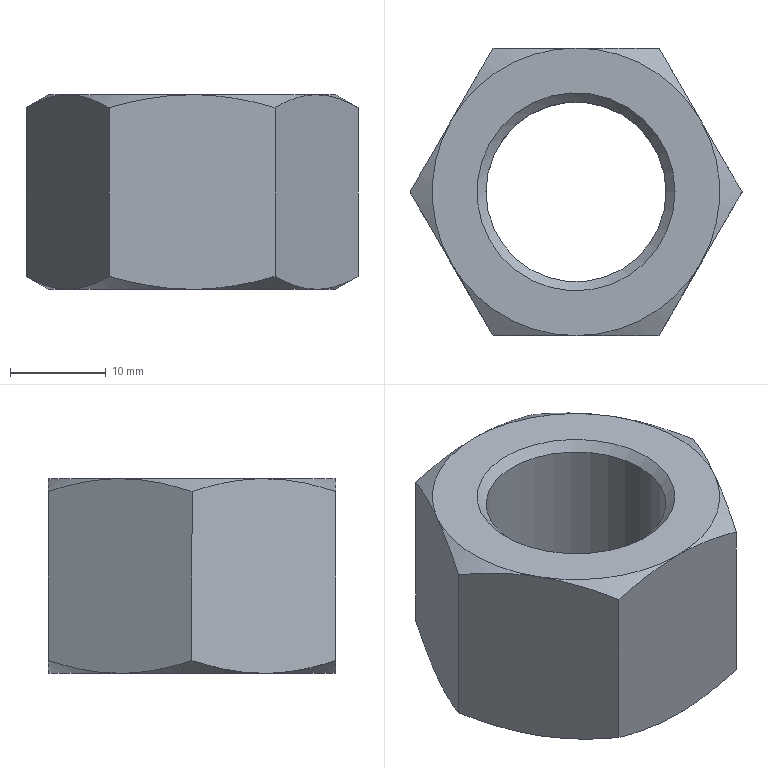Part | NX | features META 3, SKETCH 3, DATUM_CSYS 2, EXTRUDE 2, SWP104 2, CHAMFER 1, LINE 1, SYMBOLIC_THREAD 1, THREADS 1 | 1 solid | 23 faces | box 34.641 x 30 x 20.3 mm | volume 10084 mm3 | cone 14 | plane 8 | cylinder 1 | commonest cylinder face diameters 18.782 x1
STEP:
#1=CARTESIAN_POINT('',(10.33,0.,20.3));
#2=VERTEX_POINT('',#1);
#3=CARTESIAN_POINT('',(0.,0.,20.3));
#4=DIRECTION('',(0.,0.,1.));
#5=DIRECTION('',(1.,0.,0.));
#6=AXIS2_PLACEMENT_3D('',#3,#4,#5);
#7=CIRCLE('',#6,10.33);
#8=EDGE_CURVE('',#2,#2,#7,.F.);
#9=ORIENTED_EDGE('',*,*,#8,.T.);
#10=EDGE_LOOP('',(#9));
#11=FACE_BOUND('',#10,.T.);
#12=CARTESIAN_POINT('',(-12.99,7.5,20.3));
#13=VERTEX_POINT('',#12);
#14=CARTESIAN_POINT('',(0.,15.,20.3));
#15=VERTEX_POINT('',#14);
#16=CARTESIAN_POINT('',(0.,0.,20.3));
#17=DIRECTION('',(0.,0.,-1.));
#18=DIRECTION('',(-1.,0.,0.));
#19=AXIS2_PLACEMENT_3D('',#16,#17,#18);
#20=CIRCLE('',#19,15.);
#21=EDGE_CURVE('',#13,#15,#20,.T.);
#22=ORIENTED_EDGE('',*,*,#21,.F.);
#23=CARTESIAN_POINT('',(-12.99,-7.5,20.3));
#24=VERTEX_POINT('',#23);
#25=CARTESIAN_POINT('',(0.,0.,20.3));
#26=DIRECTION('',(0.,0.,-1.));
#27=DIRECTION('',(-1.,0.,0.));
#28=AXIS2_PLACEMENT_3D('',#25,#26,#27);
#29=CIRCLE('',#28,15.);
#30=EDGE_CURVE('',#24,#13,#29,.T.);
#31=ORIENTED_EDGE('',*,*,#30,.F.);
#32=CARTESIAN_POINT('',(0.,-15.,20.3));
#33=VERTEX_POINT('',#32);
#34=CARTESIAN_POINT('',(0.,0.,20.3));
#35=DIRECTION('',(0.,0.,-1.));
#36=DIRECTION('',(-1.,0.,0.));
#37=AXIS2_PLACEMENT_3D('',#34,#35,#36);
#38=CIRCLE('',#37,15.);
#39=EDGE_CURVE('',#33,#24,#38,.T.);
#40=ORIENTED_EDGE('',*,*,#39,.F.);
#41=CARTESIAN_POINT('',(12.99,-7.5,20.3));
#42=VERTEX_POINT('',#41);
#43=CARTESIAN_POINT('',(0.,0.,20.3));
#44=DIRECTION('',(0.,0.,-1.));
#45=DIRECTION('',(-1.,0.,0.));
#46=AXIS2_PLACEMENT_3D('',#43,#44,#45);
#47=CIRCLE('',#46,15.);
#48=EDGE_CURVE('',#42,#33,#47,.T.);
#49=ORIENTED_EDGE('',*,*,#48,.F.);
#50=CARTESIAN_POINT('',(12.99,7.5,20.3));
#51=VERTEX_POINT('',#50);
#52=CARTESIAN_POINT('',(0.,0.,20.3));
#53=DIRECTION('',(0.,0.,-1.));
#54=DIRECTION('',(-1.,0.,0.));
#55=AXIS2_PLACEMENT_3D('',#52,#53,#54);
#56=CIRCLE('',#55,15.);
#57=EDGE_CURVE('',#51,#42,#56,.T.);
#58=ORIENTED_EDGE('',*,*,#57,.F.);
#59=CARTESIAN_POINT('',(0.,0.,20.3));
#60=DIRECTION('',(0.,0.,-1.));
#61=DIRECTION('',(-1.,0.,0.));
#62=AXIS2_PLACEMENT_3D('',#59,#60,#61);
#63=CIRCLE('',#62,15.);
#64=EDGE_CURVE('',#15,#51,#63,.T.);
#65=ORIENTED_EDGE('',*,*,#64,.F.);
#66=EDGE_LOOP('',(#22,#31,#40,#49,#58,#65));
#67=FACE_BOUND('',#66,.T.);
#68=CARTESIAN_POINT('',(0.,30.,20.3));
#69=DIRECTION('',(0.,0.,1.));
#70=DIRECTION('',(1.,0.,0.));
#71=AXIS2_PLACEMENT_3D('',#68,#69,#70);
#72=PLANE('',#71);
#73=ADVANCED_FACE('',(#11,#67),#72,.T.);
#74=CARTESIAN_POINT('',(10.33,0.,0.));
#75=VERTEX_POINT('',#74);
#76=CARTESIAN_POINT('',(0.,0.,0.));
#77=DIRECTION('',(0.,0.,1.));
#78=DIRECTION('',(1.,0.,0.));
#79=AXIS2_PLACEMENT_3D('',#76,#77,#78);
#80=CIRCLE('',#79,10.33);
#81=EDGE_CURVE('',#75,#75,#80,.T.);
#82=ORIENTED_EDGE('',*,*,#81,.T.);
#83=EDGE_LOOP('',(#82));
#84=FACE_BOUND('',#83,.T.);
#85=CARTESIAN_POINT('',(-12.99,-7.5,0.));
#86=VERTEX_POINT('',#85);
#87=CARTESIAN_POINT('',(-12.99,7.5,0.));
#88=VERTEX_POINT('',#87);
#89=CARTESIAN_POINT('',(0.,0.,0.));
#90=DIRECTION('',(0.,0.,-1.));
#91=DIRECTION('',(-1.,0.,0.));
#92=AXIS2_PLACEMENT_3D('',#89,#90,#91);
#93=CIRCLE('',#92,15.);
#94=EDGE_CURVE('',#86,#88,#93,.T.);
#95=ORIENTED_EDGE('',*,*,#94,.T.);
#96=CARTESIAN_POINT('',(0.,15.,0.));
#97=VERTEX_POINT('',#96);
#98=CARTESIAN_POINT('',(0.,0.,0.));
#99=DIRECTION('',(0.,0.,-1.));
#100=DIRECTION('',(-1.,0.,0.));
#101=AXIS2_PLACEMENT_3D('',#98,#99,#100);
#102=CIRCLE('',#101,15.);
#103=EDGE_CURVE('',#88,#97,#102,.T.);
#104=ORIENTED_EDGE('',*,*,#103,.T.);
#105=CARTESIAN_POINT('',(12.99,7.5,0.));
#106=VERTEX_POINT('',#105);
#107=CARTESIAN_POINT('',(0.,0.,0.));
#108=DIRECTION('',(0.,0.,-1.));
#109=DIRECTION('',(-1.,0.,0.));
#110=AXIS2_PLACEMENT_3D('',#107,#108,#109);
#111=CIRCLE('',#110,15.);
#112=EDGE_CURVE('',#97,#106,#111,.T.);
#113=ORIENTED_EDGE('',*,*,#112,.T.);
#114=CARTESIAN_POINT('',(12.99,-7.5,0.));
#115=VERTEX_POINT('',#114);
#116=CARTESIAN_POINT('',(0.,0.,0.));
#117=DIRECTION('',(0.,0.,-1.));
#118=DIRECTION('',(-1.,0.,0.));
#119=AXIS2_PLACEMENT_3D('',#116,#117,#118);
#120=CIRCLE('',#119,15.);
#121=EDGE_CURVE('',#106,#115,#120,.T.);
#122=ORIENTED_EDGE('',*,*,#121,.T.);
#123=CARTESIAN_POINT('',(0.,-15.,0.));
#124=VERTEX_POINT('',#123);
#125=CARTESIAN_POINT('',(0.,0.,0.));
#126=DIRECTION('',(0.,0.,-1.));
#127=DIRECTION('',(-1.,0.,0.));
#128=AXIS2_PLACEMENT_3D('',#125,#126,#127);
#129=CIRCLE('',#128,15.);
#130=EDGE_CURVE('',#115,#124,#129,.T.);
#131=ORIENTED_EDGE('',*,*,#130,.T.);
#132=CARTESIAN_POINT('',(0.,0.,0.));
#133=DIRECTION('',(0.,0.,-1.));
#134=DIRECTION('',(-1.,0.,0.));
#135=AXIS2_PLACEMENT_3D('',#132,#133,#134);
#136=CIRCLE('',#135,15.);
#137=EDGE_CURVE('',#124,#86,#136,.T.);
#138=ORIENTED_EDGE('',*,*,#137,.T.);
#139=EDGE_LOOP('',(#95,#104,#113,#122,#131,#138));
#140=FACE_BOUND('',#139,.T.);
#141=CARTESIAN_POINT('',(0.,30.,0.));
#142=DIRECTION('',(0.,0.,1.));
#143=DIRECTION('',(1.,0.,0.));
#144=AXIS2_PLACEMENT_3D('',#141,#142,#143);
#145=PLANE('',#144);
#146=ADVANCED_FACE('',(#84,#140),#145,.F.);
#147=CARTESIAN_POINT('',(17.321,0.,18.96));
#148=VERTEX_POINT('',#147);
#149=CARTESIAN_POINT('',(17.321,0.,1.34));
#150=VERTEX_POINT('',#149);
#151=CARTESIAN_POINT('',(17.321,0.,20.3));
#152=DIRECTION('',(0.,0.,-1.));
#153=VECTOR('',#152,1000.);
#154=LINE('',#151,#153);
#155=EDGE_CURVE('',#148,#150,#154,.T.);
#156=ORIENTED_EDGE('',*,*,#155,.T.);
#157=CARTESIAN_POINT('',(17.321,0.,1.34));
#158=CARTESIAN_POINT('',(15.904,2.454,0.5218));
#159=CARTESIAN_POINT('',(14.466,4.944,0.));
#160=CARTESIAN_POINT('',(12.99,7.5,0.));
#161=B_SPLINE_CURVE_WITH_KNOTS('',3,(#157,#158,#159,#160),.UNSPECIFIED.,.F.,.F.,(4,4),(0.000000238,0.008763),.UNSPECIFIED.);
#162=EDGE_CURVE('',#150,#106,#161,.T.);
#163=ORIENTED_EDGE('',*,*,#162,.T.);
#164=CARTESIAN_POINT('',(8.66,15.,1.34));
#165=VERTEX_POINT('',#164);
#166=CARTESIAN_POINT('',(12.99,7.5,0.));
#167=CARTESIAN_POINT('',(11.52,10.046,0.));
#168=CARTESIAN_POINT('',(10.073,12.552,0.5239));
#169=CARTESIAN_POINT('',(8.66,15.,1.34));
#170=B_SPLINE_CURVE_WITH_KNOTS('',3,(#166,#167,#168,#169),.UNSPECIFIED.,.F.,.F.,(4,4),(0.008763,0.01749),.UNSPECIFIED.);
#171=EDGE_CURVE('',#106,#165,#170,.T.);
#172=ORIENTED_EDGE('',*,*,#171,.T.);
#173=CARTESIAN_POINT('',(8.66,15.,18.96));
#174=VERTEX_POINT('',#173);
#175=CARTESIAN_POINT('',(8.66,15.,20.3));
#176=DIRECTION('',(0.,0.,-1.));
#177=VECTOR('',#176,1000.);
#178=LINE('',#175,#177);
#179=EDGE_CURVE('',#174,#165,#178,.T.);
#180=ORIENTED_EDGE('',*,*,#179,.F.);
#181=CARTESIAN_POINT('',(8.66,15.,18.96));
#182=CARTESIAN_POINT('',(10.077,12.546,19.778));
#183=CARTESIAN_POINT('',(11.515,10.056,20.3));
#184=CARTESIAN_POINT('',(12.99,7.5,20.3));
#185=B_SPLINE_CURVE_WITH_KNOTS('',3,(#181,#182,#183,#184),.UNSPECIFIED.,.F.,.F.,(4,4),(0.000000238,0.008763),.UNSPECIFIED.);
#186=EDGE_CURVE('',#174,#51,#185,.T.);
#187=ORIENTED_EDGE('',*,*,#186,.T.);
#188=CARTESIAN_POINT('',(12.99,7.5,20.3));
#189=CARTESIAN_POINT('',(14.46,4.954,20.3));
#190=CARTESIAN_POINT('',(15.907,2.448,19.776));
#191=CARTESIAN_POINT('',(17.321,0.,18.96));
#192=B_SPLINE_CURVE_WITH_KNOTS('',3,(#188,#189,#190,#191),.UNSPECIFIED.,.F.,.F.,(4,4),(0.008763,0.01749),.UNSPECIFIED.);
#193=EDGE_CURVE('',#51,#148,#192,.T.);
#194=ORIENTED_EDGE('',*,*,#193,.T.);
#195=EDGE_LOOP('',(#156,#163,#172,#180,#187,#194));
#196=FACE_BOUND('',#195,.T.);
#197=CARTESIAN_POINT('',(8.66,15.,20.3));
#198=DIRECTION('',(0.866,0.5,0.));
#199=DIRECTION('',(-0.5,0.866,0.));
#200=AXIS2_PLACEMENT_3D('',#197,#198,#199);
#201=PLANE('',#200);
#202=ADVANCED_FACE('',(#196),#201,.T.);
#203=CARTESIAN_POINT('',(8.66,-15.,18.96));
#204=VERTEX_POINT('',#203);
#205=CARTESIAN_POINT('',(8.66,-15.,1.34));
#206=VERTEX_POINT('',#205);
#207=CARTESIAN_POINT('',(8.66,-15.,20.3));
#208=DIRECTION('',(0.,0.,-1.));
#209=VECTOR('',#208,1000.);
#210=LINE('',#207,#209);
#211=EDGE_CURVE('',#204,#206,#210,.T.);
#212=ORIENTED_EDGE('',*,*,#211,.T.);
#213=CARTESIAN_POINT('',(8.66,-15.,1.34));
#214=CARTESIAN_POINT('',(10.077,-12.546,0.5218));
#215=CARTESIAN_POINT('',(11.515,-10.056,0.));
#216=CARTESIAN_POINT('',(12.99,-7.5,0.));
#217=B_SPLINE_CURVE_WITH_KNOTS('',3,(#213,#214,#215,#216),.UNSPECIFIED.,.F.,.F.,(4,4),(0.000000238,0.008763),.UNSPECIFIED.);
#218=EDGE_CURVE('',#206,#115,#217,.T.);
#219=ORIENTED_EDGE('',*,*,#218,.T.);
#220=CARTESIAN_POINT('',(12.99,-7.5,0.));
#221=CARTESIAN_POINT('',(14.46,-4.954,0.));
#222=CARTESIAN_POINT('',(15.907,-2.448,0.5239));
#223=CARTESIAN_POINT('',(17.321,0.,1.34));
#224=B_SPLINE_CURVE_WITH_KNOTS('',3,(#220,#221,#222,#223),.UNSPECIFIED.,.F.,.F.,(4,4),(0.008763,0.01749),.UNSPECIFIED.);
#225=EDGE_CURVE('',#115,#150,#224,.T.);
#226=ORIENTED_EDGE('',*,*,#225,.T.);
#227=ORIENTED_EDGE('',*,*,#155,.F.);
#228=CARTESIAN_POINT('',(17.321,0.,18.96));
#229=CARTESIAN_POINT('',(15.904,-2.454,19.778));
#230=CARTESIAN_POINT('',(14.466,-4.944,20.3));
#231=CARTESIAN_POINT('',(12.99,-7.5,20.3));
#232=B_SPLINE_CURVE_WITH_KNOTS('',3,(#228,#229,#230,#231),.UNSPECIFIED.,.F.,.F.,(4,4),(0.000000238,0.008763),.UNSPECIFIED.);
#233=EDGE_CURVE('',#148,#42,#232,.T.);
#234=ORIENTED_EDGE('',*,*,#233,.T.);
#235=CARTESIAN_POINT('',(12.99,-7.5,20.3));
#236=CARTESIAN_POINT('',(11.52,-10.046,20.3));
#237=CARTESIAN_POINT('',(10.073,-12.552,19.776));
#238=CARTESIAN_POINT('',(8.66,-15.,18.96));
#239=B_SPLINE_CURVE_WITH_KNOTS('',3,(#235,#236,#237,#238),.UNSPECIFIED.,.F.,.F.,(4,4),(0.008763,0.01749),.UNSPECIFIED.);
#240=EDGE_CURVE('',#42,#204,#239,.T.);
#241=ORIENTED_EDGE('',*,*,#240,.T.);
#242=EDGE_LOOP('',(#212,#219,#226,#227,#234,#241));
#243=FACE_BOUND('',#242,.T.);
#244=CARTESIAN_POINT('',(17.321,0.,20.3));
#245=DIRECTION('',(0.866,-0.5,0.));
#246=DIRECTION('',(0.5,0.866,0.));
#247=AXIS2_PLACEMENT_3D('',#244,#245,#246);
#248=PLANE('',#247);
#249=ADVANCED_FACE('',(#243),#248,.T.);
#250=CARTESIAN_POINT('',(-8.66,-15.,18.96));
#251=VERTEX_POINT('',#250);
#252=CARTESIAN_POINT('',(-8.66,-15.,1.34));
#253=VERTEX_POINT('',#252);
#254=CARTESIAN_POINT('',(-8.66,-15.,20.3));
#255=DIRECTION('',(0.,0.,-1.));
#256=VECTOR('',#255,1000.);
#257=LINE('',#254,#256);
#258=EDGE_CURVE('',#251,#253,#257,.T.);
#259=ORIENTED_EDGE('',*,*,#258,.T.);
#260=CARTESIAN_POINT('',(-8.66,-15.,1.34));
#261=CARTESIAN_POINT('',(-5.843,-15.,0.5265));
#262=CARTESIAN_POINT('',(-2.927,-15.,0.));
#263=CARTESIAN_POINT('',(0.,-15.,0.));
#264=B_SPLINE_CURVE_WITH_KNOTS('',3,(#260,#261,#262,#263),.UNSPECIFIED.,.F.,.F.,(4,4),(0.01545,0.02421),.UNSPECIFIED.);
#265=EDGE_CURVE('',#253,#124,#264,.T.);
#266=ORIENTED_EDGE('',*,*,#265,.T.);
#267=CARTESIAN_POINT('',(0.,-15.,0.));
#268=CARTESIAN_POINT('',(2.929,-15.,0.));
#269=CARTESIAN_POINT('',(5.86,-15.,0.5313));
#270=CARTESIAN_POINT('',(8.66,-15.,1.34));
#271=B_SPLINE_CURVE_WITH_KNOTS('',3,(#267,#268,#269,#270),.UNSPECIFIED.,.F.,.F.,(4,4),(0.02421,0.03298),.UNSPECIFIED.);
#272=EDGE_CURVE('',#124,#206,#271,.T.);
#273=ORIENTED_EDGE('',*,*,#272,.T.);
#274=ORIENTED_EDGE('',*,*,#211,.F.);
#275=CARTESIAN_POINT('',(0.,-15.,20.3));
#276=CARTESIAN_POINT('',(2.929,-15.,20.3));
#277=CARTESIAN_POINT('',(5.86,-15.,19.769));
#278=CARTESIAN_POINT('',(8.66,-15.,18.96));
#279=B_SPLINE_CURVE_WITH_KNOTS('',3,(#275,#276,#277,#278),.UNSPECIFIED.,.F.,.F.,(4,4),(0.02421,0.03298),.UNSPECIFIED.);
#280=EDGE_CURVE('',#204,#33,#279,.F.);
#281=ORIENTED_EDGE('',*,*,#280,.T.);
#282=CARTESIAN_POINT('',(-8.66,-15.,18.96));
#283=CARTESIAN_POINT('',(-5.843,-15.,19.773));
#284=CARTESIAN_POINT('',(-2.927,-15.,20.3));
#285=CARTESIAN_POINT('',(0.,-15.,20.3));
#286=B_SPLINE_CURVE_WITH_KNOTS('',3,(#282,#283,#284,#285),.UNSPECIFIED.,.F.,.F.,(4,4),(0.01545,0.02421),.UNSPECIFIED.);
#287=EDGE_CURVE('',#33,#251,#286,.F.);
#288=ORIENTED_EDGE('',*,*,#287,.T.);
#289=EDGE_LOOP('',(#259,#266,#273,#274,#281,#288));
#290=FACE_BOUND('',#289,.T.);
#291=CARTESIAN_POINT('',(8.66,-15.,20.3));
#292=DIRECTION('',(0.,-1.,0.));
#293=DIRECTION('',(1.,0.,0.));
#294=AXIS2_PLACEMENT_3D('',#291,#292,#293);
#295=PLANE('',#294);
#296=ADVANCED_FACE('',(#290),#295,.T.);
#297=CARTESIAN_POINT('',(-17.321,0.,18.96));
#298=VERTEX_POINT('',#297);
#299=CARTESIAN_POINT('',(-17.321,0.,1.34));
#300=VERTEX_POINT('',#299);
#301=CARTESIAN_POINT('',(-17.321,0.,20.3));
#302=DIRECTION('',(0.,0.,-1.));
#303=VECTOR('',#302,1000.);
#304=LINE('',#301,#303);
#305=EDGE_CURVE('',#298,#300,#304,.T.);
#306=ORIENTED_EDGE('',*,*,#305,.T.);
#307=CARTESIAN_POINT('',(-17.321,0.,1.34));
#308=CARTESIAN_POINT('',(-15.904,-2.454,0.5218));
#309=CARTESIAN_POINT('',(-14.466,-4.944,0.));
#310=CARTESIAN_POINT('',(-12.99,-7.5,0.));
#311=B_SPLINE_CURVE_WITH_KNOTS('',3,(#307,#308,#309,#310),.UNSPECIFIED.,.F.,.F.,(4,4),(0.000000238,0.008763),.UNSPECIFIED.);
#312=EDGE_CURVE('',#300,#86,#311,.T.);
#313=ORIENTED_EDGE('',*,*,#312,.T.);
#314=CARTESIAN_POINT('',(-12.99,-7.5,0.));
#315=CARTESIAN_POINT('',(-11.52,-10.046,0.));
#316=CARTESIAN_POINT('',(-10.073,-12.552,0.5239));
#317=CARTESIAN_POINT('',(-8.66,-15.,1.34));
#318=B_SPLINE_CURVE_WITH_KNOTS('',3,(#314,#315,#316,#317),.UNSPECIFIED.,.F.,.F.,(4,4),(0.008763,0.01749),.UNSPECIFIED.);
#319=EDGE_CURVE('',#86,#253,#318,.T.);
#320=ORIENTED_EDGE('',*,*,#319,.T.);
#321=ORIENTED_EDGE('',*,*,#258,.F.);
#322=CARTESIAN_POINT('',(-8.66,-15.,18.96));
#323=CARTESIAN_POINT('',(-10.077,-12.546,19.778));
#324=CARTESIAN_POINT('',(-11.515,-10.056,20.3));
#325=CARTESIAN_POINT('',(-12.99,-7.5,20.3));
#326=B_SPLINE_CURVE_WITH_KNOTS('',3,(#322,#323,#324,#325),.UNSPECIFIED.,.F.,.F.,(4,4),(0.000000238,0.008763),.UNSPECIFIED.);
#327=EDGE_CURVE('',#251,#24,#326,.T.);
#328=ORIENTED_EDGE('',*,*,#327,.T.);
#329=CARTESIAN_POINT('',(-12.99,-7.5,20.3));
#330=CARTESIAN_POINT('',(-14.46,-4.954,20.3));
#331=CARTESIAN_POINT('',(-15.907,-2.448,19.776));
#332=CARTESIAN_POINT('',(-17.321,0.,18.96));
#333=B_SPLINE_CURVE_WITH_KNOTS('',3,(#329,#330,#331,#332),.UNSPECIFIED.,.F.,.F.,(4,4),(0.008763,0.01749),.UNSPECIFIED.);
#334=EDGE_CURVE('',#24,#298,#333,.T.);
#335=ORIENTED_EDGE('',*,*,#334,.T.);
#336=EDGE_LOOP('',(#306,#313,#320,#321,#328,#335));
#337=FACE_BOUND('',#336,.T.);
#338=CARTESIAN_POINT('',(-8.66,-15.,20.3));
#339=DIRECTION('',(-0.866,-0.5,0.));
#340=DIRECTION('',(0.5,-0.866,0.));
#341=AXIS2_PLACEMENT_3D('',#338,#339,#340);
#342=PLANE('',#341);
#343=ADVANCED_FACE('',(#337),#342,.T.);
#344=CARTESIAN_POINT('',(-8.66,15.,18.96));
#345=VERTEX_POINT('',#344);
#346=CARTESIAN_POINT('',(-8.66,15.,1.34));
#347=VERTEX_POINT('',#346);
#348=CARTESIAN_POINT('',(-8.66,15.,20.3));
#349=DIRECTION('',(0.,0.,-1.));
#350=VECTOR('',#349,1000.);
#351=LINE('',#348,#350);
#352=EDGE_CURVE('',#345,#347,#351,.T.);
#353=ORIENTED_EDGE('',*,*,#352,.T.);
#354=CARTESIAN_POINT('',(-8.66,15.,1.34));
#355=CARTESIAN_POINT('',(-10.077,12.546,0.5218));
#356=CARTESIAN_POINT('',(-11.515,10.056,0.));
#357=CARTESIAN_POINT('',(-12.99,7.5,0.));
#358=B_SPLINE_CURVE_WITH_KNOTS('',3,(#354,#355,#356,#357),.UNSPECIFIED.,.F.,.F.,(4,4),(0.000000238,0.008763),.UNSPECIFIED.);
#359=EDGE_CURVE('',#347,#88,#358,.T.);
#360=ORIENTED_EDGE('',*,*,#359,.T.);
#361=CARTESIAN_POINT('',(-12.99,7.5,0.));
#362=CARTESIAN_POINT('',(-14.46,4.954,0.));
#363=CARTESIAN_POINT('',(-15.907,2.448,0.5239));
#364=CARTESIAN_POINT('',(-17.321,0.,1.34));
#365=B_SPLINE_CURVE_WITH_KNOTS('',3,(#361,#362,#363,#364),.UNSPECIFIED.,.F.,.F.,(4,4),(0.008763,0.01749),.UNSPECIFIED.);
#366=EDGE_CURVE('',#88,#300,#365,.T.);
#367=ORIENTED_EDGE('',*,*,#366,.T.);
#368=ORIENTED_EDGE('',*,*,#305,.F.);
#369=CARTESIAN_POINT('',(-17.321,0.,18.96));
#370=CARTESIAN_POINT('',(-15.904,2.454,19.778));
#371=CARTESIAN_POINT('',(-14.466,4.944,20.3));
#372=CARTESIAN_POINT('',(-12.99,7.5,20.3));
#373=B_SPLINE_CURVE_WITH_KNOTS('',3,(#369,#370,#371,#372),.UNSPECIFIED.,.F.,.F.,(4,4),(0.000000238,0.008763),.UNSPECIFIED.);
#374=EDGE_CURVE('',#298,#13,#373,.T.);
#375=ORIENTED_EDGE('',*,*,#374,.T.);
#376=CARTESIAN_POINT('',(-12.99,7.5,20.3));
#377=CARTESIAN_POINT('',(-11.52,10.046,20.3));
#378=CARTESIAN_POINT('',(-10.073,12.552,19.776));
#379=CARTESIAN_POINT('',(-8.66,15.,18.96));
#380=B_SPLINE_CURVE_WITH_KNOTS('',3,(#376,#377,#378,#379),.UNSPECIFIED.,.F.,.F.,(4,4),(0.008763,0.01749),.UNSPECIFIED.);
#381=EDGE_CURVE('',#13,#345,#380,.T.);
#382=ORIENTED_EDGE('',*,*,#381,.T.);
#383=EDGE_LOOP('',(#353,#360,#367,#368,#375,#382));
#384=FACE_BOUND('',#383,.T.);
#385=CARTESIAN_POINT('',(-17.321,0.,20.3));
#386=DIRECTION('',(-0.866,0.5,0.));
#387=DIRECTION('',(-0.5,-0.866,0.));
#388=AXIS2_PLACEMENT_3D('',#385,#386,#387);
#389=PLANE('',#388);
#390=ADVANCED_FACE('',(#384),#389,.T.);
#391=ORIENTED_EDGE('',*,*,#179,.T.);
#392=CARTESIAN_POINT('',(0.,15.,0.));
#393=CARTESIAN_POINT('',(2.929,15.,0.));
#394=CARTESIAN_POINT('',(5.86,15.,0.5313));
#395=CARTESIAN_POINT('',(8.66,15.,1.34));
#396=B_SPLINE_CURVE_WITH_KNOTS('',3,(#392,#393,#394,#395),.UNSPECIFIED.,.F.,.F.,(4,4),(0.02421,0.03298),.UNSPECIFIED.);
#397=EDGE_CURVE('',#165,#97,#396,.F.);
#398=ORIENTED_EDGE('',*,*,#397,.T.);
#399=CARTESIAN_POINT('',(-8.66,15.,1.34));
#400=CARTESIAN_POINT('',(-5.843,15.,0.5265));
#401=CARTESIAN_POINT('',(-2.927,15.,0.));
#402=CARTESIAN_POINT('',(0.,15.,0.));
#403=B_SPLINE_CURVE_WITH_KNOTS('',3,(#399,#400,#401,#402),.UNSPECIFIED.,.F.,.F.,(4,4),(0.01545,0.02421),.UNSPECIFIED.);
#404=EDGE_CURVE('',#97,#347,#403,.F.);
#405=ORIENTED_EDGE('',*,*,#404,.T.);
#406=ORIENTED_EDGE('',*,*,#352,.F.);
#407=CARTESIAN_POINT('',(-8.66,15.,18.96));
#408=CARTESIAN_POINT('',(-5.843,15.,19.773));
#409=CARTESIAN_POINT('',(-2.927,15.,20.3));
#410=CARTESIAN_POINT('',(0.,15.,20.3));
#411=B_SPLINE_CURVE_WITH_KNOTS('',3,(#407,#408,#409,#410),.UNSPECIFIED.,.F.,.F.,(4,4),(0.01545,0.02421),.UNSPECIFIED.);
#412=EDGE_CURVE('',#345,#15,#411,.T.);
#413=ORIENTED_EDGE('',*,*,#412,.T.);
#414=CARTESIAN_POINT('',(0.,15.,20.3));
#415=CARTESIAN_POINT('',(2.929,15.,20.3));
#416=CARTESIAN_POINT('',(5.86,15.,19.769));
#417=CARTESIAN_POINT('',(8.66,15.,18.96));
#418=B_SPLINE_CURVE_WITH_KNOTS('',3,(#414,#415,#416,#417),.UNSPECIFIED.,.F.,.F.,(4,4),(0.02421,0.03298),.UNSPECIFIED.);
#419=EDGE_CURVE('',#15,#174,#418,.T.);
#420=ORIENTED_EDGE('',*,*,#419,.T.);
#421=EDGE_LOOP('',(#391,#398,#405,#406,#413,#420));
#422=FACE_BOUND('',#421,.T.);
#423=CARTESIAN_POINT('',(-8.66,15.,20.3));
#424=DIRECTION('',(0.,1.,0.));
#425=DIRECTION('',(0.,0.,1.));
#426=AXIS2_PLACEMENT_3D('',#423,#424,#425);
#427=PLANE('',#426);
#428=ADVANCED_FACE('',(#422),#427,.T.);
#429=ORIENTED_EDGE('',*,*,#419,.F.);
#430=ORIENTED_EDGE('',*,*,#64,.T.);
#431=ORIENTED_EDGE('',*,*,#186,.F.);
#432=EDGE_LOOP('',(#429,#430,#431));
#433=FACE_BOUND('',#432,.T.);
#434=CARTESIAN_POINT('',(0.,0.,18.96));
#435=DIRECTION('',(0.,0.,-1.));
#436=DIRECTION('',(-1.,0.,0.));
#437=AXIS2_PLACEMENT_3D('',#434,#435,#436);
#438=CONICAL_SURFACE('',#437,17.321,1.047);
#439=ADVANCED_FACE('',(#433),#438,.T.);
#440=ORIENTED_EDGE('',*,*,#21,.T.);
#441=ORIENTED_EDGE('',*,*,#412,.F.);
#442=ORIENTED_EDGE('',*,*,#381,.F.);
#443=EDGE_LOOP('',(#440,#441,#442));
#444=FACE_BOUND('',#443,.T.);
#445=CARTESIAN_POINT('',(0.,0.,18.96));
#446=DIRECTION('',(0.,0.,-1.));
#447=DIRECTION('',(-1.,0.,0.));
#448=AXIS2_PLACEMENT_3D('',#445,#446,#447);
#449=CONICAL_SURFACE('',#448,17.321,1.047);
#450=ADVANCED_FACE('',(#444),#449,.T.);
#451=ORIENTED_EDGE('',*,*,#30,.T.);
#452=ORIENTED_EDGE('',*,*,#374,.F.);
#453=ORIENTED_EDGE('',*,*,#334,.F.);
#454=EDGE_LOOP('',(#451,#452,#453));
#455=FACE_BOUND('',#454,.T.);
#456=CARTESIAN_POINT('',(0.,0.,18.96));
#457=DIRECTION('',(0.,0.,-1.));
#458=DIRECTION('',(-1.,0.,0.));
#459=AXIS2_PLACEMENT_3D('',#456,#457,#458);
#460=CONICAL_SURFACE('',#459,17.321,1.047);
#461=ADVANCED_FACE('',(#455),#460,.T.);
#462=ORIENTED_EDGE('',*,*,#39,.T.);
#463=ORIENTED_EDGE('',*,*,#327,.F.);
#464=ORIENTED_EDGE('',*,*,#287,.F.);
#465=EDGE_LOOP('',(#462,#463,#464));
#466=FACE_BOUND('',#465,.T.);
#467=CARTESIAN_POINT('',(0.,0.,18.96));
#468=DIRECTION('',(0.,0.,-1.));
#469=DIRECTION('',(-1.,0.,0.));
#470=AXIS2_PLACEMENT_3D('',#467,#468,#469);
#471=CONICAL_SURFACE('',#470,17.321,1.047);
#472=ADVANCED_FACE('',(#466),#471,.T.);
#473=ORIENTED_EDGE('',*,*,#48,.T.);
#474=ORIENTED_EDGE('',*,*,#280,.F.);
#475=ORIENTED_EDGE('',*,*,#240,.F.);
#476=EDGE_LOOP('',(#473,#474,#475));
#477=FACE_BOUND('',#476,.T.);
#478=CARTESIAN_POINT('',(0.,0.,18.96));
#479=DIRECTION('',(0.,0.,-1.));
#480=DIRECTION('',(-1.,0.,0.));
#481=AXIS2_PLACEMENT_3D('',#478,#479,#480);
#482=CONICAL_SURFACE('',#481,17.321,1.047);
#483=ADVANCED_FACE('',(#477),#482,.T.);
#484=ORIENTED_EDGE('',*,*,#57,.T.);
#485=ORIENTED_EDGE('',*,*,#233,.F.);
#486=ORIENTED_EDGE('',*,*,#193,.F.);
#487=EDGE_LOOP('',(#484,#485,#486));
#488=FACE_BOUND('',#487,.T.);
#489=CARTESIAN_POINT('',(0.,0.,18.96));
#490=DIRECTION('',(0.,0.,-1.));
#491=DIRECTION('',(-1.,0.,0.));
#492=AXIS2_PLACEMENT_3D('',#489,#490,#491);
#493=CONICAL_SURFACE('',#492,17.321,1.047);
#494=ADVANCED_FACE('',(#488),#493,.T.);
#495=ORIENTED_EDGE('',*,*,#404,.F.);
#496=ORIENTED_EDGE('',*,*,#103,.F.);
#497=ORIENTED_EDGE('',*,*,#359,.F.);
#498=EDGE_LOOP('',(#495,#496,#497));
#499=FACE_BOUND('',#498,.T.);
#500=CARTESIAN_POINT('',(0.,0.,0.));
#501=DIRECTION('',(0.,0.,1.));
#502=DIRECTION('',(1.,0.,0.));
#503=AXIS2_PLACEMENT_3D('',#500,#501,#502);
#504=CONICAL_SURFACE('',#503,15.,1.047);
#505=ADVANCED_FACE('',(#499),#504,.T.);
#506=ORIENTED_EDGE('',*,*,#112,.F.);
#507=ORIENTED_EDGE('',*,*,#397,.F.);
#508=ORIENTED_EDGE('',*,*,#171,.F.);
#509=EDGE_LOOP('',(#506,#507,#508));
#510=FACE_BOUND('',#509,.T.);
#511=CARTESIAN_POINT('',(0.,0.,0.));
#512=DIRECTION('',(0.,0.,1.));
#513=DIRECTION('',(1.,0.,0.));
#514=AXIS2_PLACEMENT_3D('',#511,#512,#513);
#515=CONICAL_SURFACE('',#514,15.,1.047);
#516=ADVANCED_FACE('',(#510),#515,.T.);
#517=ORIENTED_EDGE('',*,*,#366,.F.);
#518=ORIENTED_EDGE('',*,*,#94,.F.);
#519=ORIENTED_EDGE('',*,*,#312,.F.);
#520=EDGE_LOOP('',(#517,#518,#519));
#521=FACE_BOUND('',#520,.T.);
#522=CARTESIAN_POINT('',(0.,0.,0.));
#523=DIRECTION('',(0.,0.,1.));
#524=DIRECTION('',(1.,0.,0.));
#525=AXIS2_PLACEMENT_3D('',#522,#523,#524);
#526=CONICAL_SURFACE('',#525,15.,1.047);
#527=ADVANCED_FACE('',(#521),#526,.T.);
#528=ORIENTED_EDGE('',*,*,#319,.F.);
#529=ORIENTED_EDGE('',*,*,#137,.F.);
#530=ORIENTED_EDGE('',*,*,#265,.F.);
#531=EDGE_LOOP('',(#528,#529,#530));
#532=FACE_BOUND('',#531,.T.);
#533=CARTESIAN_POINT('',(0.,0.,0.));
#534=DIRECTION('',(0.,0.,1.));
#535=DIRECTION('',(1.,0.,0.));
#536=AXIS2_PLACEMENT_3D('',#533,#534,#535);
#537=CONICAL_SURFACE('',#536,15.,1.047);
#538=ADVANCED_FACE('',(#532),#537,.T.);
#539=ORIENTED_EDGE('',*,*,#130,.F.);
#540=ORIENTED_EDGE('',*,*,#218,.F.);
#541=ORIENTED_EDGE('',*,*,#272,.F.);
#542=EDGE_LOOP('',(#539,#540,#541));
#543=FACE_BOUND('',#542,.T.);
#544=CARTESIAN_POINT('',(0.,0.,0.));
#545=DIRECTION('',(0.,0.,1.));
#546=DIRECTION('',(1.,0.,0.));
#547=AXIS2_PLACEMENT_3D('',#544,#545,#546);
#548=CONICAL_SURFACE('',#547,15.,1.047);
#549=ADVANCED_FACE('',(#543),#548,.T.);
#550=ORIENTED_EDGE('',*,*,#121,.F.);
#551=ORIENTED_EDGE('',*,*,#162,.F.);
#552=ORIENTED_EDGE('',*,*,#225,.F.);
#553=EDGE_LOOP('',(#550,#551,#552));
#554=FACE_BOUND('',#553,.T.);
#555=CARTESIAN_POINT('',(0.,0.,0.));
#556=DIRECTION('',(0.,0.,1.));
#557=DIRECTION('',(1.,0.,0.));
#558=AXIS2_PLACEMENT_3D('',#555,#556,#557);
#559=CONICAL_SURFACE('',#558,15.,1.047);
#560=ADVANCED_FACE('',(#554),#559,.T.);
#561=CARTESIAN_POINT('',(9.391,0.,0.9391));
#562=VERTEX_POINT('',#561);
#563=CARTESIAN_POINT('',(0.,0.,0.9391));
#564=DIRECTION('',(0.,0.,1.));
#565=DIRECTION('',(1.,0.,0.));
#566=AXIS2_PLACEMENT_3D('',#563,#564,#565);
#567=CIRCLE('',#566,9.391);
#568=EDGE_CURVE('',#562,#562,#567,.F.);
#569=ORIENTED_EDGE('',*,*,#568,.T.);
#570=EDGE_LOOP('',(#569));
#571=FACE_BOUND('',#570,.T.);
#572=CARTESIAN_POINT('',(9.391,0.,19.361));
#573=VERTEX_POINT('',#572);
#574=CARTESIAN_POINT('',(0.,0.,19.361));
#575=DIRECTION('',(0.,0.,1.));
#576=DIRECTION('',(1.,0.,0.));
#577=AXIS2_PLACEMENT_3D('',#574,#575,#576);
#578=CIRCLE('',#577,9.391);
#579=EDGE_CURVE('',#573,#573,#578,.T.);
#580=ORIENTED_EDGE('',*,*,#579,.T.);
#581=EDGE_LOOP('',(#580));
#582=FACE_BOUND('',#581,.T.);
#583=CARTESIAN_POINT('',(0.,0.,20.3));
#584=DIRECTION('',(0.,0.,-1.));
#585=DIRECTION('',(-1.,0.,0.));
#586=AXIS2_PLACEMENT_3D('',#583,#584,#585);
#587=CYLINDRICAL_SURFACE('',#586,9.391);
#588=ADVANCED_FACE('',(#571,#582),#587,.F.);
#589=ORIENTED_EDGE('',*,*,#81,.F.);
#590=EDGE_LOOP('',(#589));
#591=FACE_BOUND('',#590,.T.);
#592=ORIENTED_EDGE('',*,*,#568,.F.);
#593=EDGE_LOOP('',(#592));
#594=FACE_BOUND('',#593,.T.);
#595=CARTESIAN_POINT('',(0.,0.,0.9391));
#596=DIRECTION('',(0.,0.,-1.));
#597=DIRECTION('',(-1.,0.,0.));
#598=AXIS2_PLACEMENT_3D('',#595,#596,#597);
#599=CONICAL_SURFACE('',#598,9.391,0.7854);
#600=ADVANCED_FACE('',(#591,#594),#599,.F.);
#601=ORIENTED_EDGE('',*,*,#579,.F.);
#602=EDGE_LOOP('',(#601));
#603=FACE_BOUND('',#602,.T.);
#604=ORIENTED_EDGE('',*,*,#8,.F.);
#605=EDGE_LOOP('',(#604));
#606=FACE_BOUND('',#605,.T.);
#607=CARTESIAN_POINT('',(0.,0.,20.3));
#608=DIRECTION('',(0.,0.,1.));
#609=DIRECTION('',(1.,0.,0.));
#610=AXIS2_PLACEMENT_3D('',#607,#608,#609);
#611=CONICAL_SURFACE('',#610,10.33,0.7854);
#612=ADVANCED_FACE('',(#603,#606),#611,.F.);
#613=CLOSED_SHELL('',(#73,#146,#202,#249,#296,#343,#390,#428,#439,#450,#461,#472,#483,#494,#505,#516,#527,#538,#549,#560,#588,#600,#612));
#614=MANIFOLD_SOLID_BREP('',#613);
#615=(LENGTH_UNIT()NAMED_UNIT(*)SI_UNIT(.MILLI.,.METRE.));
#616=UNCERTAINTY_MEASURE_WITH_UNIT(LENGTH_MEASURE(0.0508),#615,'','');
#617=(NAMED_UNIT(*)PLANE_ANGLE_UNIT()SI_UNIT($,.RADIAN.));
#618=(NAMED_UNIT(*)SI_UNIT($,.STERADIAN.)SOLID_ANGLE_UNIT());
#619=(GEOMETRIC_REPRESENTATION_CONTEXT(3)GLOBAL_UNCERTAINTY_ASSIGNED_CONTEXT((#616))GLOBAL_UNIT_ASSIGNED_CONTEXT((#615,#617,#618))REPRESENTATION_CONTEXT('',''));
#620=ADVANCED_BREP_SHAPE_REPRESENTATION('',(#614),#619);